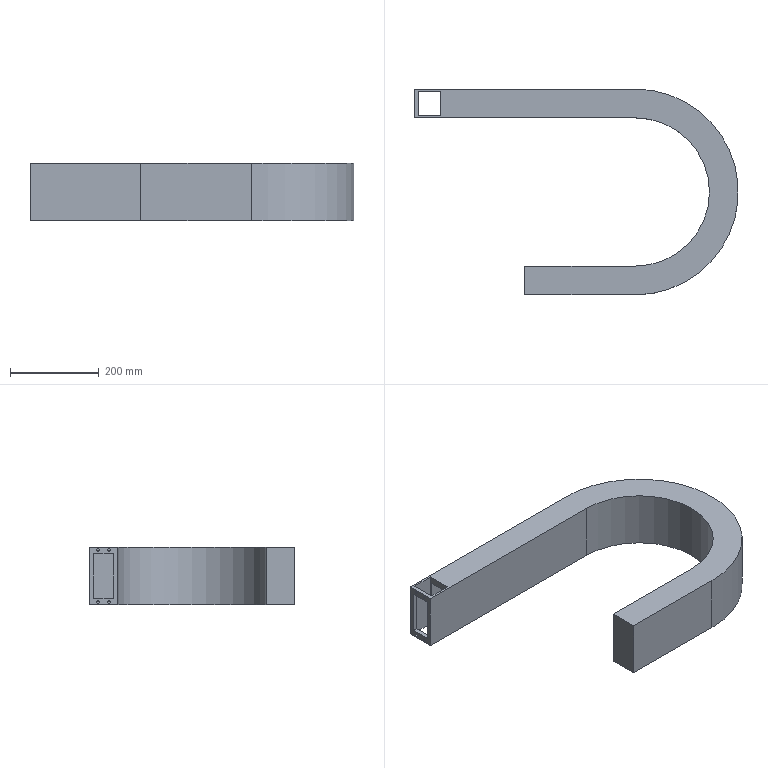Part | SolidWorks | features ICE 3, Extrusion 1 | 1 solid | 31 faces | box 732.5 x 465 x 130 mm | volume 10613161 mm3 | plane 21 | cylinder 10 | commonest cylinder face diameters 6 x8 335 x1 465 x1
STEP:
#1=CARTESIAN_POINT('',(-940.428,254.022,9.));
#2=VERTEX_POINT('',#1);
#3=CARTESIAN_POINT('',(-940.428,254.022,3.));
#4=VERTEX_POINT('',#3);
#5=CARTESIAN_POINT('',(-940.428,254.022,6.));
#6=DIRECTION('',(1.,0.,0.));
#7=DIRECTION('',(0.,0.,1.));
#8=AXIS2_PLACEMENT_3D('',#5,#6,#7);
#9=CIRCLE('',#8,3.);
#10=EDGE_CURVE('',#2,#4,#9,.T.);
#11=ORIENTED_EDGE('',*,*,#10,.T.);
#12=CARTESIAN_POINT('',(-950.428,254.022,3.));
#13=VERTEX_POINT('',#12);
#14=CARTESIAN_POINT('',(-930.428,254.022,3.));
#15=DIRECTION('',(-1.,0.,0.));
#16=VECTOR('',#15,1000.);
#17=LINE('',#14,#16);
#18=EDGE_CURVE('',#4,#13,#17,.T.);
#19=ORIENTED_EDGE('',*,*,#18,.T.);
#20=CARTESIAN_POINT('',(-950.428,254.022,9.));
#21=VERTEX_POINT('',#20);
#22=CARTESIAN_POINT('',(-950.428,254.022,6.));
#23=DIRECTION('',(-1.,0.,0.));
#24=DIRECTION('',(0.,0.,1.));
#25=AXIS2_PLACEMENT_3D('',#22,#23,#24);
#26=CIRCLE('',#25,3.);
#27=EDGE_CURVE('',#13,#21,#26,.T.);
#28=ORIENTED_EDGE('',*,*,#27,.T.);
#29=CARTESIAN_POINT('',(-930.428,254.022,9.));
#30=DIRECTION('',(-1.,0.,0.));
#31=VECTOR('',#30,1000.);
#32=LINE('',#29,#31);
#33=EDGE_CURVE('',#2,#21,#32,.T.);
#34=ORIENTED_EDGE('',*,*,#33,.F.);
#35=EDGE_LOOP('',(#11,#19,#28,#34));
#36=FACE_OUTER_BOUND('',#35,.T.);
#37=CARTESIAN_POINT('',(-930.428,254.022,6.));
#38=DIRECTION('',(-1.,0.,0.));
#39=DIRECTION('',(0.,0.,1.));
#40=AXIS2_PLACEMENT_3D('',#37,#38,#39);
#41=CYLINDRICAL_SURFACE('',#40,3.);
#42=ADVANCED_FACE('',(#36),#41,.F.);
#43=CARTESIAN_POINT('',(-940.428,279.022,127.));
#44=VERTEX_POINT('',#43);
#45=CARTESIAN_POINT('',(-940.428,279.022,121.));
#46=VERTEX_POINT('',#45);
#47=CARTESIAN_POINT('',(-940.428,279.022,124.));
#48=DIRECTION('',(1.,0.,0.));
#49=DIRECTION('',(0.,0.,1.));
#50=AXIS2_PLACEMENT_3D('',#47,#48,#49);
#51=CIRCLE('',#50,3.);
#52=EDGE_CURVE('',#44,#46,#51,.T.);
#53=ORIENTED_EDGE('',*,*,#52,.T.);
#54=CARTESIAN_POINT('',(-950.428,279.022,121.));
#55=VERTEX_POINT('',#54);
#56=CARTESIAN_POINT('',(-930.428,279.022,121.));
#57=DIRECTION('',(-1.,0.,0.));
#58=VECTOR('',#57,1000.);
#59=LINE('',#56,#58);
#60=EDGE_CURVE('',#46,#55,#59,.T.);
#61=ORIENTED_EDGE('',*,*,#60,.T.);
#62=CARTESIAN_POINT('',(-950.428,279.022,127.));
#63=VERTEX_POINT('',#62);
#64=CARTESIAN_POINT('',(-950.428,279.022,124.));
#65=DIRECTION('',(-1.,0.,0.));
#66=DIRECTION('',(0.,0.,1.));
#67=AXIS2_PLACEMENT_3D('',#64,#65,#66);
#68=CIRCLE('',#67,3.);
#69=EDGE_CURVE('',#55,#63,#68,.T.);
#70=ORIENTED_EDGE('',*,*,#69,.T.);
#71=CARTESIAN_POINT('',(-930.428,279.022,127.));
#72=DIRECTION('',(-1.,0.,0.));
#73=VECTOR('',#72,1000.);
#74=LINE('',#71,#73);
#75=EDGE_CURVE('',#44,#63,#74,.T.);
#76=ORIENTED_EDGE('',*,*,#75,.F.);
#77=EDGE_LOOP('',(#53,#61,#70,#76));
#78=FACE_OUTER_BOUND('',#77,.T.);
#79=CARTESIAN_POINT('',(-930.428,279.022,124.));
#80=DIRECTION('',(-1.,0.,0.));
#81=DIRECTION('',(0.,0.,1.));
#82=AXIS2_PLACEMENT_3D('',#79,#80,#81);
#83=CYLINDRICAL_SURFACE('',#82,3.);
#84=ADVANCED_FACE('',(#78),#83,.F.);
#85=CARTESIAN_POINT('',(-940.428,254.022,127.));
#86=VERTEX_POINT('',#85);
#87=CARTESIAN_POINT('',(-940.428,254.022,121.));
#88=VERTEX_POINT('',#87);
#89=CARTESIAN_POINT('',(-940.428,254.022,124.));
#90=DIRECTION('',(1.,0.,0.));
#91=DIRECTION('',(0.,0.,1.));
#92=AXIS2_PLACEMENT_3D('',#89,#90,#91);
#93=CIRCLE('',#92,3.);
#94=EDGE_CURVE('',#86,#88,#93,.T.);
#95=ORIENTED_EDGE('',*,*,#94,.T.);
#96=CARTESIAN_POINT('',(-950.428,254.022,121.));
#97=VERTEX_POINT('',#96);
#98=CARTESIAN_POINT('',(-930.428,254.022,121.));
#99=DIRECTION('',(-1.,0.,0.));
#100=VECTOR('',#99,1000.);
#101=LINE('',#98,#100);
#102=EDGE_CURVE('',#88,#97,#101,.T.);
#103=ORIENTED_EDGE('',*,*,#102,.T.);
#104=CARTESIAN_POINT('',(-950.428,254.022,127.));
#105=VERTEX_POINT('',#104);
#106=CARTESIAN_POINT('',(-950.428,254.022,124.));
#107=DIRECTION('',(-1.,0.,0.));
#108=DIRECTION('',(0.,0.,1.));
#109=AXIS2_PLACEMENT_3D('',#106,#107,#108);
#110=CIRCLE('',#109,3.);
#111=EDGE_CURVE('',#97,#105,#110,.T.);
#112=ORIENTED_EDGE('',*,*,#111,.T.);
#113=CARTESIAN_POINT('',(-930.428,254.022,127.));
#114=DIRECTION('',(-1.,0.,0.));
#115=VECTOR('',#114,1000.);
#116=LINE('',#113,#115);
#117=EDGE_CURVE('',#86,#105,#116,.T.);
#118=ORIENTED_EDGE('',*,*,#117,.F.);
#119=EDGE_LOOP('',(#95,#103,#112,#118));
#120=FACE_OUTER_BOUND('',#119,.T.);
#121=CARTESIAN_POINT('',(-930.428,254.022,124.));
#122=DIRECTION('',(-1.,0.,0.));
#123=DIRECTION('',(0.,0.,1.));
#124=AXIS2_PLACEMENT_3D('',#121,#122,#123);
#125=CYLINDRICAL_SURFACE('',#124,3.);
#126=ADVANCED_FACE('',(#120),#125,.F.);
#127=CARTESIAN_POINT('',(-940.428,279.022,9.));
#128=VERTEX_POINT('',#127);
#129=CARTESIAN_POINT('',(-940.428,279.022,3.));
#130=VERTEX_POINT('',#129);
#131=CARTESIAN_POINT('',(-940.428,279.022,6.));
#132=DIRECTION('',(1.,0.,0.));
#133=DIRECTION('',(0.,0.,1.));
#134=AXIS2_PLACEMENT_3D('',#131,#132,#133);
#135=CIRCLE('',#134,3.);
#136=EDGE_CURVE('',#128,#130,#135,.T.);
#137=ORIENTED_EDGE('',*,*,#136,.T.);
#138=CARTESIAN_POINT('',(-950.428,279.022,3.));
#139=VERTEX_POINT('',#138);
#140=CARTESIAN_POINT('',(-930.428,279.022,3.));
#141=DIRECTION('',(-1.,0.,0.));
#142=VECTOR('',#141,1000.);
#143=LINE('',#140,#142);
#144=EDGE_CURVE('',#130,#139,#143,.T.);
#145=ORIENTED_EDGE('',*,*,#144,.T.);
#146=CARTESIAN_POINT('',(-950.428,279.022,9.));
#147=VERTEX_POINT('',#146);
#148=CARTESIAN_POINT('',(-950.428,279.022,6.));
#149=DIRECTION('',(-1.,0.,0.));
#150=DIRECTION('',(0.,0.,1.));
#151=AXIS2_PLACEMENT_3D('',#148,#149,#150);
#152=CIRCLE('',#151,3.);
#153=EDGE_CURVE('',#139,#147,#152,.T.);
#154=ORIENTED_EDGE('',*,*,#153,.T.);
#155=CARTESIAN_POINT('',(-930.428,279.022,9.));
#156=DIRECTION('',(-1.,0.,0.));
#157=VECTOR('',#156,1000.);
#158=LINE('',#155,#157);
#159=EDGE_CURVE('',#128,#147,#158,.T.);
#160=ORIENTED_EDGE('',*,*,#159,.F.);
#161=EDGE_LOOP('',(#137,#145,#154,#160));
#162=FACE_OUTER_BOUND('',#161,.T.);
#163=CARTESIAN_POINT('',(-930.428,279.022,6.));
#164=DIRECTION('',(-1.,0.,0.));
#165=DIRECTION('',(0.,0.,1.));
#166=AXIS2_PLACEMENT_3D('',#163,#164,#165);
#167=CYLINDRICAL_SURFACE('',#166,3.);
#168=ADVANCED_FACE('',(#162),#167,.F.);
#169=CARTESIAN_POINT('',(-450.428,-165.978,0.));
#170=VERTEX_POINT('',#169);
#171=CARTESIAN_POINT('',(-450.428,299.022,0.));
#172=VERTEX_POINT('',#171);
#173=CARTESIAN_POINT('',(-450.428,66.522,0.));
#174=DIRECTION('',(0.,0.,1.));
#175=DIRECTION('',(1.,0.,0.));
#176=AXIS2_PLACEMENT_3D('',#173,#174,#175);
#177=CIRCLE('',#176,232.5);
#178=EDGE_CURVE('',#170,#172,#177,.T.);
#179=ORIENTED_EDGE('',*,*,#178,.T.);
#180=CARTESIAN_POINT('',(-450.428,299.022,130.));
#181=VERTEX_POINT('',#180);
#182=CARTESIAN_POINT('',(-450.428,299.022,130.));
#183=DIRECTION('',(0.,0.,-1.));
#184=VECTOR('',#183,1000.);
#185=LINE('',#182,#184);
#186=EDGE_CURVE('',#181,#172,#185,.T.);
#187=ORIENTED_EDGE('',*,*,#186,.F.);
#188=CARTESIAN_POINT('',(-450.428,-165.978,130.));
#189=VERTEX_POINT('',#188);
#190=CARTESIAN_POINT('',(-450.428,66.522,130.));
#191=DIRECTION('',(0.,0.,1.));
#192=DIRECTION('',(1.,0.,0.));
#193=AXIS2_PLACEMENT_3D('',#190,#191,#192);
#194=CIRCLE('',#193,232.5);
#195=EDGE_CURVE('',#189,#181,#194,.T.);
#196=ORIENTED_EDGE('',*,*,#195,.F.);
#197=CARTESIAN_POINT('',(-450.428,-165.978,130.));
#198=DIRECTION('',(0.,0.,-1.));
#199=VECTOR('',#198,1000.);
#200=LINE('',#197,#199);
#201=EDGE_CURVE('',#189,#170,#200,.T.);
#202=ORIENTED_EDGE('',*,*,#201,.T.);
#203=EDGE_LOOP('',(#179,#187,#196,#202));
#204=FACE_OUTER_BOUND('',#203,.T.);
#205=CARTESIAN_POINT('',(-450.428,66.522,130.));
#206=DIRECTION('',(0.,0.,-1.));
#207=DIRECTION('',(-1.,0.,0.));
#208=AXIS2_PLACEMENT_3D('',#205,#206,#207);
#209=CYLINDRICAL_SURFACE('',#208,232.5);
#210=ADVANCED_FACE('',(#204),#209,.T.);
#211=CARTESIAN_POINT('',(-950.428,299.022,0.));
#212=VERTEX_POINT('',#211);
#213=CARTESIAN_POINT('',(-450.428,299.022,0.));
#214=DIRECTION('',(-1.,0.,0.));
#215=VECTOR('',#214,1000.);
#216=LINE('',#213,#215);
#217=EDGE_CURVE('',#172,#212,#216,.T.);
#218=ORIENTED_EDGE('',*,*,#217,.T.);
#219=CARTESIAN_POINT('',(-950.428,299.022,130.));
#220=VERTEX_POINT('',#219);
#221=CARTESIAN_POINT('',(-950.428,299.022,130.));
#222=DIRECTION('',(0.,0.,-1.));
#223=VECTOR('',#222,1000.);
#224=LINE('',#221,#223);
#225=EDGE_CURVE('',#220,#212,#224,.T.);
#226=ORIENTED_EDGE('',*,*,#225,.F.);
#227=CARTESIAN_POINT('',(-450.428,299.022,130.));
#228=DIRECTION('',(-1.,0.,0.));
#229=VECTOR('',#228,1000.);
#230=LINE('',#227,#229);
#231=EDGE_CURVE('',#181,#220,#230,.T.);
#232=ORIENTED_EDGE('',*,*,#231,.F.);
#233=ORIENTED_EDGE('',*,*,#186,.T.);
#234=EDGE_LOOP('',(#218,#226,#232,#233));
#235=FACE_OUTER_BOUND('',#234,.T.);
#236=CARTESIAN_POINT('',(-450.428,299.022,130.));
#237=DIRECTION('',(0.,-1.,0.));
#238=DIRECTION('',(1.,0.,0.));
#239=AXIS2_PLACEMENT_3D('',#236,#237,#238);
#240=PLANE('',#239);
#241=ADVANCED_FACE('',(#235),#240,.F.);
#242=CARTESIAN_POINT('',(-950.428,244.022,15.));
#243=VERTEX_POINT('',#242);
#244=CARTESIAN_POINT('',(-950.428,244.022,115.));
#245=VERTEX_POINT('',#244);
#246=CARTESIAN_POINT('',(-950.428,244.022,15.));
#247=DIRECTION('',(0.,0.,1.));
#248=VECTOR('',#247,1000.);
#249=LINE('',#246,#248);
#250=EDGE_CURVE('',#243,#245,#249,.T.);
#251=ORIENTED_EDGE('',*,*,#250,.F.);
#252=CARTESIAN_POINT('',(-950.428,289.022,15.));
#253=VERTEX_POINT('',#252);
#254=CARTESIAN_POINT('',(-950.428,289.022,15.));
#255=DIRECTION('',(0.,-1.,0.));
#256=VECTOR('',#255,1000.);
#257=LINE('',#254,#256);
#258=EDGE_CURVE('',#253,#243,#257,.T.);
#259=ORIENTED_EDGE('',*,*,#258,.F.);
#260=CARTESIAN_POINT('',(-950.428,289.022,115.));
#261=VERTEX_POINT('',#260);
#262=CARTESIAN_POINT('',(-950.428,289.022,15.));
#263=DIRECTION('',(0.,0.,-1.));
#264=VECTOR('',#263,1000.);
#265=LINE('',#262,#264);
#266=EDGE_CURVE('',#261,#253,#265,.T.);
#267=ORIENTED_EDGE('',*,*,#266,.F.);
#268=CARTESIAN_POINT('',(-950.428,289.022,115.));
#269=DIRECTION('',(0.,1.,0.));
#270=VECTOR('',#269,1000.);
#271=LINE('',#268,#270);
#272=EDGE_CURVE('',#245,#261,#271,.T.);
#273=ORIENTED_EDGE('',*,*,#272,.F.);
#274=EDGE_LOOP('',(#251,#259,#267,#273));
#275=FACE_BOUND('',#274,.T.);
#276=CARTESIAN_POINT('',(-950.428,254.022,6.));
#277=DIRECTION('',(-1.,0.,0.));
#278=DIRECTION('',(0.,0.,1.));
#279=AXIS2_PLACEMENT_3D('',#276,#277,#278);
#280=CIRCLE('',#279,3.);
#281=EDGE_CURVE('',#21,#13,#280,.T.);
#282=ORIENTED_EDGE('',*,*,#281,.F.);
#283=ORIENTED_EDGE('',*,*,#27,.F.);
#284=EDGE_LOOP('',(#282,#283));
#285=FACE_BOUND('',#284,.T.);
#286=CARTESIAN_POINT('',(-950.428,279.022,124.));
#287=DIRECTION('',(-1.,0.,0.));
#288=DIRECTION('',(0.,0.,1.));
#289=AXIS2_PLACEMENT_3D('',#286,#287,#288);
#290=CIRCLE('',#289,3.);
#291=EDGE_CURVE('',#63,#55,#290,.T.);
#292=ORIENTED_EDGE('',*,*,#291,.F.);
#293=ORIENTED_EDGE('',*,*,#69,.F.);
#294=EDGE_LOOP('',(#292,#293));
#295=FACE_BOUND('',#294,.T.);
#296=CARTESIAN_POINT('',(-950.428,254.022,124.));
#297=DIRECTION('',(-1.,0.,0.));
#298=DIRECTION('',(0.,0.,1.));
#299=AXIS2_PLACEMENT_3D('',#296,#297,#298);
#300=CIRCLE('',#299,3.);
#301=EDGE_CURVE('',#105,#97,#300,.T.);
#302=ORIENTED_EDGE('',*,*,#301,.F.);
#303=ORIENTED_EDGE('',*,*,#111,.F.);
#304=EDGE_LOOP('',(#302,#303));
#305=FACE_BOUND('',#304,.T.);
#306=CARTESIAN_POINT('',(-950.428,279.022,6.));
#307=DIRECTION('',(-1.,0.,0.));
#308=DIRECTION('',(0.,0.,1.));
#309=AXIS2_PLACEMENT_3D('',#306,#307,#308);
#310=CIRCLE('',#309,3.);
#311=EDGE_CURVE('',#147,#139,#310,.T.);
#312=ORIENTED_EDGE('',*,*,#311,.F.);
#313=ORIENTED_EDGE('',*,*,#153,.F.);
#314=EDGE_LOOP('',(#312,#313));
#315=FACE_BOUND('',#314,.T.);
#316=CARTESIAN_POINT('',(-950.428,234.022,0.));
#317=VERTEX_POINT('',#316);
#318=CARTESIAN_POINT('',(-950.428,299.022,0.));
#319=DIRECTION('',(0.,-1.,0.));
#320=VECTOR('',#319,1000.);
#321=LINE('',#318,#320);
#322=EDGE_CURVE('',#212,#317,#321,.T.);
#323=ORIENTED_EDGE('',*,*,#322,.T.);
#324=CARTESIAN_POINT('',(-950.428,234.022,130.));
#325=VERTEX_POINT('',#324);
#326=CARTESIAN_POINT('',(-950.428,234.022,130.));
#327=DIRECTION('',(0.,0.,-1.));
#328=VECTOR('',#327,1000.);
#329=LINE('',#326,#328);
#330=EDGE_CURVE('',#325,#317,#329,.T.);
#331=ORIENTED_EDGE('',*,*,#330,.F.);
#332=CARTESIAN_POINT('',(-950.428,299.022,130.));
#333=DIRECTION('',(0.,-1.,0.));
#334=VECTOR('',#333,1000.);
#335=LINE('',#332,#334);
#336=EDGE_CURVE('',#220,#325,#335,.T.);
#337=ORIENTED_EDGE('',*,*,#336,.F.);
#338=ORIENTED_EDGE('',*,*,#225,.T.);
#339=EDGE_LOOP('',(#323,#331,#337,#338));
#340=FACE_OUTER_BOUND('',#339,.T.);
#341=CARTESIAN_POINT('',(-950.428,299.022,130.));
#342=DIRECTION('',(1.,0.,0.));
#343=DIRECTION('',(0.,0.,-1.));
#344=AXIS2_PLACEMENT_3D('',#341,#342,#343);
#345=PLANE('',#344);
#346=ADVANCED_FACE('',(#275,#285,#295,#305,#315,#340),#345,.F.);
#347=CARTESIAN_POINT('',(-450.428,234.022,0.));
#348=VERTEX_POINT('',#347);
#349=CARTESIAN_POINT('',(-450.428,234.022,0.));
#350=DIRECTION('',(1.,0.,0.));
#351=VECTOR('',#350,1000.);
#352=LINE('',#349,#351);
#353=EDGE_CURVE('',#317,#348,#352,.T.);
#354=ORIENTED_EDGE('',*,*,#353,.T.);
#355=CARTESIAN_POINT('',(-450.428,234.022,130.));
#356=VERTEX_POINT('',#355);
#357=CARTESIAN_POINT('',(-450.428,234.022,130.));
#358=DIRECTION('',(0.,0.,-1.));
#359=VECTOR('',#358,1000.);
#360=LINE('',#357,#359);
#361=EDGE_CURVE('',#356,#348,#360,.T.);
#362=ORIENTED_EDGE('',*,*,#361,.F.);
#363=CARTESIAN_POINT('',(-450.428,234.022,130.));
#364=DIRECTION('',(1.,0.,0.));
#365=VECTOR('',#364,1000.);
#366=LINE('',#363,#365);
#367=EDGE_CURVE('',#325,#356,#366,.T.);
#368=ORIENTED_EDGE('',*,*,#367,.F.);
#369=ORIENTED_EDGE('',*,*,#330,.T.);
#370=EDGE_LOOP('',(#354,#362,#368,#369));
#371=FACE_OUTER_BOUND('',#370,.T.);
#372=CARTESIAN_POINT('',(-450.428,234.022,130.));
#373=DIRECTION('',(0.,1.,0.));
#374=DIRECTION('',(-1.,0.,0.));
#375=AXIS2_PLACEMENT_3D('',#372,#373,#374);
#376=PLANE('',#375);
#377=ADVANCED_FACE('',(#371),#376,.F.);
#378=CARTESIAN_POINT('',(-450.428,-100.978,0.));
#379=VERTEX_POINT('',#378);
#380=CARTESIAN_POINT('',(-450.428,66.522,0.));
#381=DIRECTION('',(0.,0.,-1.));
#382=DIRECTION('',(1.,0.,0.));
#383=AXIS2_PLACEMENT_3D('',#380,#381,#382);
#384=CIRCLE('',#383,167.5);
#385=EDGE_CURVE('',#348,#379,#384,.T.);
#386=ORIENTED_EDGE('',*,*,#385,.T.);
#387=CARTESIAN_POINT('',(-450.428,-100.978,130.));
#388=VERTEX_POINT('',#387);
#389=CARTESIAN_POINT('',(-450.428,-100.978,130.));
#390=DIRECTION('',(0.,0.,-1.));
#391=VECTOR('',#390,1000.);
#392=LINE('',#389,#391);
#393=EDGE_CURVE('',#388,#379,#392,.T.);
#394=ORIENTED_EDGE('',*,*,#393,.F.);
#395=CARTESIAN_POINT('',(-450.428,66.522,130.));
#396=DIRECTION('',(0.,0.,-1.));
#397=DIRECTION('',(1.,0.,0.));
#398=AXIS2_PLACEMENT_3D('',#395,#396,#397);
#399=CIRCLE('',#398,167.5);
#400=EDGE_CURVE('',#356,#388,#399,.T.);
#401=ORIENTED_EDGE('',*,*,#400,.F.);
#402=ORIENTED_EDGE('',*,*,#361,.T.);
#403=EDGE_LOOP('',(#386,#394,#401,#402));
#404=FACE_OUTER_BOUND('',#403,.T.);
#405=CARTESIAN_POINT('',(-450.428,66.522,130.));
#406=DIRECTION('',(0.,0.,-1.));
#407=DIRECTION('',(-1.,0.,0.));
#408=AXIS2_PLACEMENT_3D('',#405,#406,#407);
#409=CYLINDRICAL_SURFACE('',#408,167.5);
#410=ADVANCED_FACE('',(#404),#409,.F.);
#411=CARTESIAN_POINT('',(-700.428,-100.978,0.));
#412=VERTEX_POINT('',#411);
#413=CARTESIAN_POINT('',(-450.428,-100.978,0.));
#414=DIRECTION('',(-1.,0.,0.));
#415=VECTOR('',#414,1000.);
#416=LINE('',#413,#415);
#417=EDGE_CURVE('',#379,#412,#416,.T.);
#418=ORIENTED_EDGE('',*,*,#417,.T.);
#419=CARTESIAN_POINT('',(-700.428,-100.978,130.));
#420=VERTEX_POINT('',#419);
#421=CARTESIAN_POINT('',(-700.428,-100.978,130.));
#422=DIRECTION('',(0.,0.,-1.));
#423=VECTOR('',#422,1000.);
#424=LINE('',#421,#423);
#425=EDGE_CURVE('',#420,#412,#424,.T.);
#426=ORIENTED_EDGE('',*,*,#425,.F.);
#427=CARTESIAN_POINT('',(-450.428,-100.978,130.));
#428=DIRECTION('',(-1.,0.,0.));
#429=VECTOR('',#428,1000.);
#430=LINE('',#427,#429);
#431=EDGE_CURVE('',#388,#420,#430,.T.);
#432=ORIENTED_EDGE('',*,*,#431,.F.);
#433=ORIENTED_EDGE('',*,*,#393,.T.);
#434=EDGE_LOOP('',(#418,#426,#432,#433));
#435=FACE_OUTER_BOUND('',#434,.T.);
#436=CARTESIAN_POINT('',(-450.428,-100.978,130.));
#437=DIRECTION('',(0.,-1.,0.));
#438=DIRECTION('',(1.,0.,0.));
#439=AXIS2_PLACEMENT_3D('',#436,#437,#438);
#440=PLANE('',#439);
#441=ADVANCED_FACE('',(#435),#440,.F.);
#442=CARTESIAN_POINT('',(-700.428,-165.978,0.));
#443=VERTEX_POINT('',#442);
#444=CARTESIAN_POINT('',(-700.428,-165.978,0.));
#445=DIRECTION('',(0.,-1.,0.));
#446=VECTOR('',#445,1000.);
#447=LINE('',#444,#446);
#448=EDGE_CURVE('',#412,#443,#447,.T.);
#449=ORIENTED_EDGE('',*,*,#448,.T.);
#450=CARTESIAN_POINT('',(-700.428,-165.978,130.));
#451=VERTEX_POINT('',#450);
#452=CARTESIAN_POINT('',(-700.428,-165.978,130.));
#453=DIRECTION('',(0.,0.,-1.));
#454=VECTOR('',#453,1000.);
#455=LINE('',#452,#454);
#456=EDGE_CURVE('',#451,#443,#455,.T.);
#457=ORIENTED_EDGE('',*,*,#456,.F.);
#458=CARTESIAN_POINT('',(-700.428,-165.978,130.));
#459=DIRECTION('',(0.,-1.,0.));
#460=VECTOR('',#459,1000.);
#461=LINE('',#458,#460);
#462=EDGE_CURVE('',#420,#451,#461,.T.);
#463=ORIENTED_EDGE('',*,*,#462,.F.);
#464=ORIENTED_EDGE('',*,*,#425,.T.);
#465=EDGE_LOOP('',(#449,#457,#463,#464));
#466=FACE_OUTER_BOUND('',#465,.T.);
#467=CARTESIAN_POINT('',(-700.428,-165.978,130.));
#468=DIRECTION('',(1.,0.,0.));
#469=DIRECTION('',(0.,0.,-1.));
#470=AXIS2_PLACEMENT_3D('',#467,#468,#469);
#471=PLANE('',#470);
#472=ADVANCED_FACE('',(#466),#471,.F.);
#473=CARTESIAN_POINT('',(-450.428,-165.978,0.));
#474=DIRECTION('',(1.,0.,0.));
#475=VECTOR('',#474,1000.);
#476=LINE('',#473,#475);
#477=EDGE_CURVE('',#443,#170,#476,.T.);
#478=ORIENTED_EDGE('',*,*,#477,.T.);
#479=ORIENTED_EDGE('',*,*,#201,.F.);
#480=CARTESIAN_POINT('',(-450.428,-165.978,130.));
#481=DIRECTION('',(1.,0.,0.));
#482=VECTOR('',#481,1000.);
#483=LINE('',#480,#482);
#484=EDGE_CURVE('',#451,#189,#483,.T.);
#485=ORIENTED_EDGE('',*,*,#484,.F.);
#486=ORIENTED_EDGE('',*,*,#456,.T.);
#487=EDGE_LOOP('',(#478,#479,#485,#486));
#488=FACE_OUTER_BOUND('',#487,.T.);
#489=CARTESIAN_POINT('',(-450.428,-165.978,130.));
#490=DIRECTION('',(0.,1.,0.));
#491=DIRECTION('',(-1.,0.,0.));
#492=AXIS2_PLACEMENT_3D('',#489,#490,#491);
#493=PLANE('',#492);
#494=ADVANCED_FACE('',(#488),#493,.F.);
#495=CARTESIAN_POINT('',(-940.428,294.022,130.));
#496=VERTEX_POINT('',#495);
#497=CARTESIAN_POINT('',(-940.428,239.022,130.));
#498=VERTEX_POINT('',#497);
#499=CARTESIAN_POINT('',(-940.428,294.022,130.));
#500=DIRECTION('',(0.,-1.,0.));
#501=VECTOR('',#500,1000.);
#502=LINE('',#499,#501);
#503=EDGE_CURVE('',#496,#498,#502,.T.);
#504=ORIENTED_EDGE('',*,*,#503,.F.);
#505=CARTESIAN_POINT('',(-890.428,294.022,130.));
#506=VERTEX_POINT('',#505);
#507=CARTESIAN_POINT('',(-940.428,294.022,130.));
#508=DIRECTION('',(-1.,0.,0.));
#509=VECTOR('',#508,1000.);
#510=LINE('',#507,#509);
#511=EDGE_CURVE('',#506,#496,#510,.T.);
#512=ORIENTED_EDGE('',*,*,#511,.F.);
#513=CARTESIAN_POINT('',(-890.428,239.022,130.));
#514=VERTEX_POINT('',#513);
#515=CARTESIAN_POINT('',(-890.428,294.022,130.));
#516=DIRECTION('',(0.,1.,0.));
#517=VECTOR('',#516,1000.);
#518=LINE('',#515,#517);
#519=EDGE_CURVE('',#514,#506,#518,.T.);
#520=ORIENTED_EDGE('',*,*,#519,.F.);
#521=CARTESIAN_POINT('',(-940.428,239.022,130.));
#522=DIRECTION('',(1.,0.,0.));
#523=VECTOR('',#522,1000.);
#524=LINE('',#521,#523);
#525=EDGE_CURVE('',#498,#514,#524,.T.);
#526=ORIENTED_EDGE('',*,*,#525,.F.);
#527=EDGE_LOOP('',(#504,#512,#520,#526));
#528=FACE_BOUND('',#527,.T.);
#529=ORIENTED_EDGE('',*,*,#195,.T.);
#530=ORIENTED_EDGE('',*,*,#231,.T.);
#531=ORIENTED_EDGE('',*,*,#336,.T.);
#532=ORIENTED_EDGE('',*,*,#367,.T.);
#533=ORIENTED_EDGE('',*,*,#400,.T.);
#534=ORIENTED_EDGE('',*,*,#431,.T.);
#535=ORIENTED_EDGE('',*,*,#462,.T.);
#536=ORIENTED_EDGE('',*,*,#484,.T.);
#537=EDGE_LOOP('',(#529,#530,#531,#532,#533,#534,#535,#536));
#538=FACE_OUTER_BOUND('',#537,.T.);
#539=CARTESIAN_POINT('',(-450.428,66.522,130.));
#540=DIRECTION('',(0.,0.,1.));
#541=DIRECTION('',(1.,0.,0.));
#542=AXIS2_PLACEMENT_3D('',#539,#540,#541);
#543=PLANE('',#542);
#544=ADVANCED_FACE('',(#528,#538),#543,.T.);
#545=CARTESIAN_POINT('',(-890.428,294.022,0.));
#546=VERTEX_POINT('',#545);
#547=CARTESIAN_POINT('',(-940.428,294.022,0.));
#548=VERTEX_POINT('',#547);
#549=CARTESIAN_POINT('',(-450.428,294.022,0.));
#550=DIRECTION('',(-1.,0.,0.));
#551=VECTOR('',#550,1000.);
#552=LINE('',#549,#551);
#553=EDGE_CURVE('',#546,#548,#552,.T.);
#554=ORIENTED_EDGE('',*,*,#553,.T.);
#555=CARTESIAN_POINT('',(-940.428,239.022,0.));
#556=VERTEX_POINT('',#555);
#557=CARTESIAN_POINT('',(-940.428,66.522,0.));
#558=DIRECTION('',(0.,-1.,0.));
#559=VECTOR('',#558,1000.);
#560=LINE('',#557,#559);
#561=EDGE_CURVE('',#548,#556,#560,.T.);
#562=ORIENTED_EDGE('',*,*,#561,.T.);
#563=CARTESIAN_POINT('',(-890.428,239.022,0.));
#564=VERTEX_POINT('',#563);
#565=CARTESIAN_POINT('',(-450.428,239.022,0.));
#566=DIRECTION('',(1.,0.,0.));
#567=VECTOR('',#566,1000.);
#568=LINE('',#565,#567);
#569=EDGE_CURVE('',#556,#564,#568,.T.);
#570=ORIENTED_EDGE('',*,*,#569,.T.);
#571=CARTESIAN_POINT('',(-890.428,66.522,0.));
#572=DIRECTION('',(0.,1.,0.));
#573=VECTOR('',#572,1000.);
#574=LINE('',#571,#573);
#575=EDGE_CURVE('',#564,#546,#574,.T.);
#576=ORIENTED_EDGE('',*,*,#575,.T.);
#577=EDGE_LOOP('',(#554,#562,#570,#576));
#578=FACE_BOUND('',#577,.T.);
#579=ORIENTED_EDGE('',*,*,#178,.F.);
#580=ORIENTED_EDGE('',*,*,#477,.F.);
#581=ORIENTED_EDGE('',*,*,#448,.F.);
#582=ORIENTED_EDGE('',*,*,#417,.F.);
#583=ORIENTED_EDGE('',*,*,#385,.F.);
#584=ORIENTED_EDGE('',*,*,#353,.F.);
#585=ORIENTED_EDGE('',*,*,#322,.F.);
#586=ORIENTED_EDGE('',*,*,#217,.F.);
#587=EDGE_LOOP('',(#579,#580,#581,#582,#583,#584,#585,#586));
#588=FACE_OUTER_BOUND('',#587,.T.);
#589=CARTESIAN_POINT('',(-450.428,66.522,0.));
#590=DIRECTION('',(0.,0.,1.));
#591=DIRECTION('',(1.,0.,0.));
#592=AXIS2_PLACEMENT_3D('',#589,#590,#591);
#593=PLANE('',#592);
#594=ADVANCED_FACE('',(#578,#588),#593,.F.);
#595=ORIENTED_EDGE('',*,*,#144,.F.);
#596=CARTESIAN_POINT('',(-940.428,279.022,6.));
#597=DIRECTION('',(1.,0.,0.));
#598=DIRECTION('',(0.,0.,1.));
#599=AXIS2_PLACEMENT_3D('',#596,#597,#598);
#600=CIRCLE('',#599,3.);
#601=EDGE_CURVE('',#130,#128,#600,.T.);
#602=ORIENTED_EDGE('',*,*,#601,.T.);
#603=ORIENTED_EDGE('',*,*,#159,.T.);
#604=ORIENTED_EDGE('',*,*,#311,.T.);
#605=EDGE_LOOP('',(#595,#602,#603,#604));
#606=FACE_OUTER_BOUND('',#605,.T.);
#607=CARTESIAN_POINT('',(-930.428,279.022,6.));
#608=DIRECTION('',(-1.,0.,0.));
#609=DIRECTION('',(0.,0.,1.));
#610=AXIS2_PLACEMENT_3D('',#607,#608,#609);
#611=CYLINDRICAL_SURFACE('',#610,3.);
#612=ADVANCED_FACE('',(#606),#611,.F.);
#613=ORIENTED_EDGE('',*,*,#102,.F.);
#614=CARTESIAN_POINT('',(-940.428,254.022,124.));
#615=DIRECTION('',(1.,0.,0.));
#616=DIRECTION('',(0.,0.,1.));
#617=AXIS2_PLACEMENT_3D('',#614,#615,#616);
#618=CIRCLE('',#617,3.);
#619=EDGE_CURVE('',#88,#86,#618,.T.);
#620=ORIENTED_EDGE('',*,*,#619,.T.);
#621=ORIENTED_EDGE('',*,*,#117,.T.);
#622=ORIENTED_EDGE('',*,*,#301,.T.);
#623=EDGE_LOOP('',(#613,#620,#621,#622));
#624=FACE_OUTER_BOUND('',#623,.T.);
#625=CARTESIAN_POINT('',(-930.428,254.022,124.));
#626=DIRECTION('',(-1.,0.,0.));
#627=DIRECTION('',(0.,0.,1.));
#628=AXIS2_PLACEMENT_3D('',#625,#626,#627);
#629=CYLINDRICAL_SURFACE('',#628,3.);
#630=ADVANCED_FACE('',(#624),#629,.F.);
#631=ORIENTED_EDGE('',*,*,#60,.F.);
#632=CARTESIAN_POINT('',(-940.428,279.022,124.));
#633=DIRECTION('',(1.,0.,0.));
#634=DIRECTION('',(0.,0.,1.));
#635=AXIS2_PLACEMENT_3D('',#632,#633,#634);
#636=CIRCLE('',#635,3.);
#637=EDGE_CURVE('',#46,#44,#636,.T.);
#638=ORIENTED_EDGE('',*,*,#637,.T.);
#639=ORIENTED_EDGE('',*,*,#75,.T.);
#640=ORIENTED_EDGE('',*,*,#291,.T.);
#641=EDGE_LOOP('',(#631,#638,#639,#640));
#642=FACE_OUTER_BOUND('',#641,.T.);
#643=CARTESIAN_POINT('',(-930.428,279.022,124.));
#644=DIRECTION('',(-1.,0.,0.));
#645=DIRECTION('',(0.,0.,1.));
#646=AXIS2_PLACEMENT_3D('',#643,#644,#645);
#647=CYLINDRICAL_SURFACE('',#646,3.);
#648=ADVANCED_FACE('',(#642),#647,.F.);
#649=ORIENTED_EDGE('',*,*,#18,.F.);
#650=CARTESIAN_POINT('',(-940.428,254.022,6.));
#651=DIRECTION('',(1.,0.,0.));
#652=DIRECTION('',(0.,0.,1.));
#653=AXIS2_PLACEMENT_3D('',#650,#651,#652);
#654=CIRCLE('',#653,3.);
#655=EDGE_CURVE('',#4,#2,#654,.T.);
#656=ORIENTED_EDGE('',*,*,#655,.T.);
#657=ORIENTED_EDGE('',*,*,#33,.T.);
#658=ORIENTED_EDGE('',*,*,#281,.T.);
#659=EDGE_LOOP('',(#649,#656,#657,#658));
#660=FACE_OUTER_BOUND('',#659,.T.);
#661=CARTESIAN_POINT('',(-930.428,254.022,6.));
#662=DIRECTION('',(-1.,0.,0.));
#663=DIRECTION('',(0.,0.,1.));
#664=AXIS2_PLACEMENT_3D('',#661,#662,#663);
#665=CYLINDRICAL_SURFACE('',#664,3.);
#666=ADVANCED_FACE('',(#660),#665,.F.);
#667=CARTESIAN_POINT('',(-890.428,294.022,-20.));
#668=DIRECTION('',(0.,0.,1.));
#669=VECTOR('',#668,1000.);
#670=LINE('',#667,#669);
#671=EDGE_CURVE('',#546,#506,#670,.T.);
#672=ORIENTED_EDGE('',*,*,#671,.T.);
#673=ORIENTED_EDGE('',*,*,#511,.T.);
#674=CARTESIAN_POINT('',(-940.428,294.022,-20.));
#675=DIRECTION('',(0.,0.,1.));
#676=VECTOR('',#675,1000.);
#677=LINE('',#674,#676);
#678=EDGE_CURVE('',#548,#496,#677,.T.);
#679=ORIENTED_EDGE('',*,*,#678,.F.);
#680=ORIENTED_EDGE('',*,*,#553,.F.);
#681=EDGE_LOOP('',(#672,#673,#679,#680));
#682=FACE_OUTER_BOUND('',#681,.T.);
#683=CARTESIAN_POINT('',(-940.428,294.022,-20.));
#684=DIRECTION('',(0.,1.,0.));
#685=DIRECTION('',(0.,0.,1.));
#686=AXIS2_PLACEMENT_3D('',#683,#684,#685);
#687=PLANE('',#686);
#688=ADVANCED_FACE('',(#682),#687,.F.);
#689=CARTESIAN_POINT('',(-890.428,244.022,115.));
#690=VERTEX_POINT('',#689);
#691=CARTESIAN_POINT('',(-890.428,244.022,15.));
#692=VERTEX_POINT('',#691);
#693=CARTESIAN_POINT('',(-890.428,244.022,-20.));
#694=DIRECTION('',(0.,0.,-1.));
#695=VECTOR('',#694,1000.);
#696=LINE('',#693,#695);
#697=EDGE_CURVE('',#690,#692,#696,.T.);
#698=ORIENTED_EDGE('',*,*,#697,.T.);
#699=CARTESIAN_POINT('',(-890.428,289.022,15.));
#700=VERTEX_POINT('',#699);
#701=CARTESIAN_POINT('',(-890.428,294.022,15.));
#702=DIRECTION('',(0.,1.,0.));
#703=VECTOR('',#702,1000.);
#704=LINE('',#701,#703);
#705=EDGE_CURVE('',#692,#700,#704,.T.);
#706=ORIENTED_EDGE('',*,*,#705,.T.);
#707=CARTESIAN_POINT('',(-890.428,289.022,115.));
#708=VERTEX_POINT('',#707);
#709=CARTESIAN_POINT('',(-890.428,289.022,-20.));
#710=DIRECTION('',(0.,0.,1.));
#711=VECTOR('',#710,1000.);
#712=LINE('',#709,#711);
#713=EDGE_CURVE('',#700,#708,#712,.T.);
#714=ORIENTED_EDGE('',*,*,#713,.T.);
#715=CARTESIAN_POINT('',(-890.428,294.022,115.));
#716=DIRECTION('',(0.,-1.,0.));
#717=VECTOR('',#716,1000.);
#718=LINE('',#715,#717);
#719=EDGE_CURVE('',#708,#690,#718,.T.);
#720=ORIENTED_EDGE('',*,*,#719,.T.);
#721=EDGE_LOOP('',(#698,#706,#714,#720));
#722=FACE_BOUND('',#721,.T.);
#723=CARTESIAN_POINT('',(-890.428,239.022,-20.));
#724=DIRECTION('',(0.,0.,1.));
#725=VECTOR('',#724,1000.);
#726=LINE('',#723,#725);
#727=EDGE_CURVE('',#564,#514,#726,.T.);
#728=ORIENTED_EDGE('',*,*,#727,.T.);
#729=ORIENTED_EDGE('',*,*,#519,.T.);
#730=ORIENTED_EDGE('',*,*,#671,.F.);
#731=ORIENTED_EDGE('',*,*,#575,.F.);
#732=EDGE_LOOP('',(#728,#729,#730,#731));
#733=FACE_OUTER_BOUND('',#732,.T.);
#734=CARTESIAN_POINT('',(-890.428,294.022,-20.));
#735=DIRECTION('',(1.,0.,0.));
#736=DIRECTION('',(0.,0.,-1.));
#737=AXIS2_PLACEMENT_3D('',#734,#735,#736);
#738=PLANE('',#737);
#739=ADVANCED_FACE('',(#722,#733),#738,.F.);
#740=CARTESIAN_POINT('',(-940.428,239.022,-20.));
#741=DIRECTION('',(0.,0.,1.));
#742=VECTOR('',#741,1000.);
#743=LINE('',#740,#742);
#744=EDGE_CURVE('',#556,#498,#743,.T.);
#745=ORIENTED_EDGE('',*,*,#744,.T.);
#746=ORIENTED_EDGE('',*,*,#525,.T.);
#747=ORIENTED_EDGE('',*,*,#727,.F.);
#748=ORIENTED_EDGE('',*,*,#569,.F.);
#749=EDGE_LOOP('',(#745,#746,#747,#748));
#750=FACE_OUTER_BOUND('',#749,.T.);
#751=CARTESIAN_POINT('',(-940.428,239.022,-20.));
#752=DIRECTION('',(0.,-1.,0.));
#753=DIRECTION('',(0.,0.,-1.));
#754=AXIS2_PLACEMENT_3D('',#751,#752,#753);
#755=PLANE('',#754);
#756=ADVANCED_FACE('',(#750),#755,.F.);
#757=CARTESIAN_POINT('',(-940.428,289.022,115.));
#758=VERTEX_POINT('',#757);
#759=CARTESIAN_POINT('',(-940.428,289.022,15.));
#760=VERTEX_POINT('',#759);
#761=CARTESIAN_POINT('',(-940.428,289.022,-20.));
#762=DIRECTION('',(0.,0.,-1.));
#763=VECTOR('',#762,1000.);
#764=LINE('',#761,#763);
#765=EDGE_CURVE('',#758,#760,#764,.T.);
#766=ORIENTED_EDGE('',*,*,#765,.T.);
#767=CARTESIAN_POINT('',(-940.428,244.022,15.));
#768=VERTEX_POINT('',#767);
#769=CARTESIAN_POINT('',(-940.428,294.022,15.));
#770=DIRECTION('',(0.,-1.,0.));
#771=VECTOR('',#770,1000.);
#772=LINE('',#769,#771);
#773=EDGE_CURVE('',#760,#768,#772,.T.);
#774=ORIENTED_EDGE('',*,*,#773,.T.);
#775=CARTESIAN_POINT('',(-940.428,244.022,115.));
#776=VERTEX_POINT('',#775);
#777=CARTESIAN_POINT('',(-940.428,244.022,-20.));
#778=DIRECTION('',(0.,0.,1.));
#779=VECTOR('',#778,1000.);
#780=LINE('',#777,#779);
#781=EDGE_CURVE('',#768,#776,#780,.T.);
#782=ORIENTED_EDGE('',*,*,#781,.T.);
#783=CARTESIAN_POINT('',(-940.428,294.022,115.));
#784=DIRECTION('',(0.,1.,0.));
#785=VECTOR('',#784,1000.);
#786=LINE('',#783,#785);
#787=EDGE_CURVE('',#776,#758,#786,.T.);
#788=ORIENTED_EDGE('',*,*,#787,.T.);
#789=EDGE_LOOP('',(#766,#774,#782,#788));
#790=FACE_BOUND('',#789,.T.);
#791=ORIENTED_EDGE('',*,*,#94,.F.);
#792=ORIENTED_EDGE('',*,*,#619,.F.);
#793=EDGE_LOOP('',(#791,#792));
#794=FACE_BOUND('',#793,.T.);
#795=ORIENTED_EDGE('',*,*,#10,.F.);
#796=ORIENTED_EDGE('',*,*,#655,.F.);
#797=EDGE_LOOP('',(#795,#796));
#798=FACE_BOUND('',#797,.T.);
#799=ORIENTED_EDGE('',*,*,#52,.F.);
#800=ORIENTED_EDGE('',*,*,#637,.F.);
#801=EDGE_LOOP('',(#799,#800));
#802=FACE_BOUND('',#801,.T.);
#803=ORIENTED_EDGE('',*,*,#136,.F.);
#804=ORIENTED_EDGE('',*,*,#601,.F.);
#805=EDGE_LOOP('',(#803,#804));
#806=FACE_BOUND('',#805,.T.);
#807=ORIENTED_EDGE('',*,*,#678,.T.);
#808=ORIENTED_EDGE('',*,*,#503,.T.);
#809=ORIENTED_EDGE('',*,*,#744,.F.);
#810=ORIENTED_EDGE('',*,*,#561,.F.);
#811=EDGE_LOOP('',(#807,#808,#809,#810));
#812=FACE_OUTER_BOUND('',#811,.T.);
#813=CARTESIAN_POINT('',(-940.428,294.022,-20.));
#814=DIRECTION('',(-1.,0.,0.));
#815=DIRECTION('',(0.,0.,1.));
#816=AXIS2_PLACEMENT_3D('',#813,#814,#815);
#817=PLANE('',#816);
#818=ADVANCED_FACE('',(#790,#794,#798,#802,#806,#812),#817,.F.);
#819=CARTESIAN_POINT('',(-750.428,244.022,15.));
#820=DIRECTION('',(-1.,0.,0.));
#821=VECTOR('',#820,1000.);
#822=LINE('',#819,#821);
#823=EDGE_CURVE('',#768,#243,#822,.T.);
#824=ORIENTED_EDGE('',*,*,#823,.T.);
#825=ORIENTED_EDGE('',*,*,#250,.T.);
#826=CARTESIAN_POINT('',(-750.428,244.022,115.));
#827=DIRECTION('',(-1.,0.,0.));
#828=VECTOR('',#827,1000.);
#829=LINE('',#826,#828);
#830=EDGE_CURVE('',#776,#245,#829,.T.);
#831=ORIENTED_EDGE('',*,*,#830,.F.);
#832=ORIENTED_EDGE('',*,*,#781,.F.);
#833=EDGE_LOOP('',(#824,#825,#831,#832));
#834=FACE_OUTER_BOUND('',#833,.T.);
#835=CARTESIAN_POINT('',(-750.428,244.022,15.));
#836=DIRECTION('',(0.,-1.,0.));
#837=DIRECTION('',(0.,0.,-1.));
#838=AXIS2_PLACEMENT_3D('',#835,#836,#837);
#839=PLANE('',#838);
#840=ADVANCED_FACE('',(#834),#839,.F.);
#841=ORIENTED_EDGE('',*,*,#830,.T.);
#842=ORIENTED_EDGE('',*,*,#272,.T.);
#843=CARTESIAN_POINT('',(-750.428,289.022,115.));
#844=DIRECTION('',(-1.,0.,0.));
#845=VECTOR('',#844,1000.);
#846=LINE('',#843,#845);
#847=EDGE_CURVE('',#758,#261,#846,.T.);
#848=ORIENTED_EDGE('',*,*,#847,.F.);
#849=ORIENTED_EDGE('',*,*,#787,.F.);
#850=EDGE_LOOP('',(#841,#842,#848,#849));
#851=FACE_OUTER_BOUND('',#850,.T.);
#852=CARTESIAN_POINT('',(-750.428,289.022,115.));
#853=DIRECTION('',(0.,0.,1.));
#854=DIRECTION('',(0.,-1.,0.));
#855=AXIS2_PLACEMENT_3D('',#852,#853,#854);
#856=PLANE('',#855);
#857=ADVANCED_FACE('',(#851),#856,.F.);
#858=ORIENTED_EDGE('',*,*,#847,.T.);
#859=ORIENTED_EDGE('',*,*,#266,.T.);
#860=CARTESIAN_POINT('',(-750.428,289.022,15.));
#861=DIRECTION('',(-1.,0.,0.));
#862=VECTOR('',#861,1000.);
#863=LINE('',#860,#862);
#864=EDGE_CURVE('',#760,#253,#863,.T.);
#865=ORIENTED_EDGE('',*,*,#864,.F.);
#866=ORIENTED_EDGE('',*,*,#765,.F.);
#867=EDGE_LOOP('',(#858,#859,#865,#866));
#868=FACE_OUTER_BOUND('',#867,.T.);
#869=CARTESIAN_POINT('',(-750.428,289.022,15.));
#870=DIRECTION('',(0.,1.,0.));
#871=DIRECTION('',(0.,0.,1.));
#872=AXIS2_PLACEMENT_3D('',#869,#870,#871);
#873=PLANE('',#872);
#874=ADVANCED_FACE('',(#868),#873,.F.);
#875=ORIENTED_EDGE('',*,*,#864,.T.);
#876=ORIENTED_EDGE('',*,*,#258,.T.);
#877=ORIENTED_EDGE('',*,*,#823,.F.);
#878=ORIENTED_EDGE('',*,*,#773,.F.);
#879=EDGE_LOOP('',(#875,#876,#877,#878));
#880=FACE_OUTER_BOUND('',#879,.T.);
#881=CARTESIAN_POINT('',(-750.428,289.022,15.));
#882=DIRECTION('',(0.,0.,-1.));
#883=DIRECTION('',(0.,1.,0.));
#884=AXIS2_PLACEMENT_3D('',#881,#882,#883);
#885=PLANE('',#884);
#886=ADVANCED_FACE('',(#880),#885,.F.);
#887=CARTESIAN_POINT('',(-750.428,244.022,15.));
#888=VERTEX_POINT('',#887);
#889=CARTESIAN_POINT('',(-750.428,244.022,15.));
#890=DIRECTION('',(-1.,0.,0.));
#891=VECTOR('',#890,1000.);
#892=LINE('',#889,#891);
#893=EDGE_CURVE('',#888,#692,#892,.T.);
#894=ORIENTED_EDGE('',*,*,#893,.F.);
#895=CARTESIAN_POINT('',(-750.428,289.022,15.));
#896=VERTEX_POINT('',#895);
#897=CARTESIAN_POINT('',(-750.428,289.022,15.));
#898=DIRECTION('',(0.,-1.,0.));
#899=VECTOR('',#898,1000.);
#900=LINE('',#897,#899);
#901=EDGE_CURVE('',#896,#888,#900,.T.);
#902=ORIENTED_EDGE('',*,*,#901,.F.);
#903=CARTESIAN_POINT('',(-750.428,289.022,15.));
#904=DIRECTION('',(-1.,0.,0.));
#905=VECTOR('',#904,1000.);
#906=LINE('',#903,#905);
#907=EDGE_CURVE('',#896,#700,#906,.T.);
#908=ORIENTED_EDGE('',*,*,#907,.T.);
#909=ORIENTED_EDGE('',*,*,#705,.F.);
#910=EDGE_LOOP('',(#894,#902,#908,#909));
#911=FACE_OUTER_BOUND('',#910,.T.);
#912=CARTESIAN_POINT('',(-750.428,289.022,15.));
#913=DIRECTION('',(0.,0.,-1.));
#914=DIRECTION('',(0.,1.,0.));
#915=AXIS2_PLACEMENT_3D('',#912,#913,#914);
#916=PLANE('',#915);
#917=ADVANCED_FACE('',(#911),#916,.F.);
#918=ORIENTED_EDGE('',*,*,#907,.F.);
#919=CARTESIAN_POINT('',(-750.428,289.022,115.));
#920=VERTEX_POINT('',#919);
#921=CARTESIAN_POINT('',(-750.428,289.022,15.));
#922=DIRECTION('',(0.,0.,-1.));
#923=VECTOR('',#922,1000.);
#924=LINE('',#921,#923);
#925=EDGE_CURVE('',#920,#896,#924,.T.);
#926=ORIENTED_EDGE('',*,*,#925,.F.);
#927=CARTESIAN_POINT('',(-750.428,289.022,115.));
#928=DIRECTION('',(-1.,0.,0.));
#929=VECTOR('',#928,1000.);
#930=LINE('',#927,#929);
#931=EDGE_CURVE('',#920,#708,#930,.T.);
#932=ORIENTED_EDGE('',*,*,#931,.T.);
#933=ORIENTED_EDGE('',*,*,#713,.F.);
#934=EDGE_LOOP('',(#918,#926,#932,#933));
#935=FACE_OUTER_BOUND('',#934,.T.);
#936=CARTESIAN_POINT('',(-750.428,289.022,15.));
#937=DIRECTION('',(0.,1.,0.));
#938=DIRECTION('',(0.,0.,1.));
#939=AXIS2_PLACEMENT_3D('',#936,#937,#938);
#940=PLANE('',#939);
#941=ADVANCED_FACE('',(#935),#940,.F.);
#942=ORIENTED_EDGE('',*,*,#931,.F.);
#943=CARTESIAN_POINT('',(-750.428,244.022,115.));
#944=VERTEX_POINT('',#943);
#945=CARTESIAN_POINT('',(-750.428,289.022,115.));
#946=DIRECTION('',(0.,1.,0.));
#947=VECTOR('',#946,1000.);
#948=LINE('',#945,#947);
#949=EDGE_CURVE('',#944,#920,#948,.T.);
#950=ORIENTED_EDGE('',*,*,#949,.F.);
#951=CARTESIAN_POINT('',(-750.428,244.022,115.));
#952=DIRECTION('',(-1.,0.,0.));
#953=VECTOR('',#952,1000.);
#954=LINE('',#951,#953);
#955=EDGE_CURVE('',#944,#690,#954,.T.);
#956=ORIENTED_EDGE('',*,*,#955,.T.);
#957=ORIENTED_EDGE('',*,*,#719,.F.);
#958=EDGE_LOOP('',(#942,#950,#956,#957));
#959=FACE_OUTER_BOUND('',#958,.T.);
#960=CARTESIAN_POINT('',(-750.428,289.022,115.));
#961=DIRECTION('',(0.,0.,1.));
#962=DIRECTION('',(0.,-1.,0.));
#963=AXIS2_PLACEMENT_3D('',#960,#961,#962);
#964=PLANE('',#963);
#965=ADVANCED_FACE('',(#959),#964,.F.);
#966=ORIENTED_EDGE('',*,*,#955,.F.);
#967=CARTESIAN_POINT('',(-750.428,244.022,15.));
#968=DIRECTION('',(0.,0.,1.));
#969=VECTOR('',#968,1000.);
#970=LINE('',#967,#969);
#971=EDGE_CURVE('',#888,#944,#970,.T.);
#972=ORIENTED_EDGE('',*,*,#971,.F.);
#973=ORIENTED_EDGE('',*,*,#893,.T.);
#974=ORIENTED_EDGE('',*,*,#697,.F.);
#975=EDGE_LOOP('',(#966,#972,#973,#974));
#976=FACE_OUTER_BOUND('',#975,.T.);
#977=CARTESIAN_POINT('',(-750.428,244.022,15.));
#978=DIRECTION('',(0.,-1.,0.));
#979=DIRECTION('',(0.,0.,-1.));
#980=AXIS2_PLACEMENT_3D('',#977,#978,#979);
#981=PLANE('',#980);
#982=ADVANCED_FACE('',(#976),#981,.F.);
#983=ORIENTED_EDGE('',*,*,#901,.T.);
#984=ORIENTED_EDGE('',*,*,#971,.T.);
#985=ORIENTED_EDGE('',*,*,#949,.T.);
#986=ORIENTED_EDGE('',*,*,#925,.T.);
#987=EDGE_LOOP('',(#983,#984,#985,#986));
#988=FACE_OUTER_BOUND('',#987,.T.);
#989=CARTESIAN_POINT('',(-750.428,0.,0.));
#990=DIRECTION('',(-1.,0.,0.));
#991=DIRECTION('',(0.,0.,1.));
#992=AXIS2_PLACEMENT_3D('',#989,#990,#991);
#993=PLANE('',#992);
#994=ADVANCED_FACE('',(#988),#993,.T.);
#995=CLOSED_SHELL('',(#42,#84,#126,#168,#210,#241,#346,#377,#410,#441,#472,#494,#544,#594,#612,#630,#648,#666,#688,#739,#756,#818,#840,#857,#874,#886,#917,#941,#965,#982,#994));
#996=MANIFOLD_SOLID_BREP('',#995);
#997=CARTESIAN_POINT('',(0.,0.,0.));
#998=DIRECTION('',(0.,0.,1.));
#999=DIRECTION('',(1.,0.,0.));
#1000=AXIS2_PLACEMENT_3D('',#997,#998,#999);
#1001=(LENGTH_UNIT()NAMED_UNIT(*)SI_UNIT(.MILLI.,.METRE.));
#1002=UNCERTAINTY_MEASURE_WITH_UNIT(LENGTH_MEASURE(0.00001),#1001,'','');
#1003=(NAMED_UNIT(*)PLANE_ANGLE_UNIT()SI_UNIT($,.RADIAN.));
#1004=(NAMED_UNIT(*)SI_UNIT($,.STERADIAN.)SOLID_ANGLE_UNIT());
#1005=(GEOMETRIC_REPRESENTATION_CONTEXT(3)GLOBAL_UNCERTAINTY_ASSIGNED_CONTEXT((#1002))GLOBAL_UNIT_ASSIGNED_CONTEXT((#1001,#1003,#1004))REPRESENTATION_CONTEXT('',''));
#1006=ADVANCED_BREP_SHAPE_REPRESENTATION('',(#996,#1000),#1005);